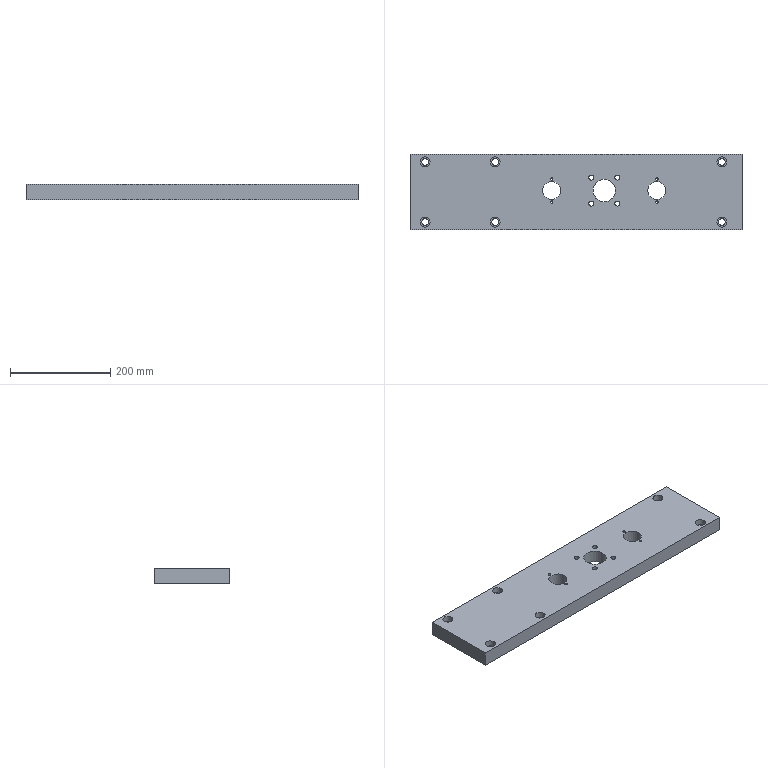Part | NX | features plate 2 | 1 solid | 44 faces | volume 2805404 mm3 | cylinder 27 | plane 17 | commonest cylinder face diameters 13.5 x6 20 x6 5 x4 10 x4 25 x4 36 x2